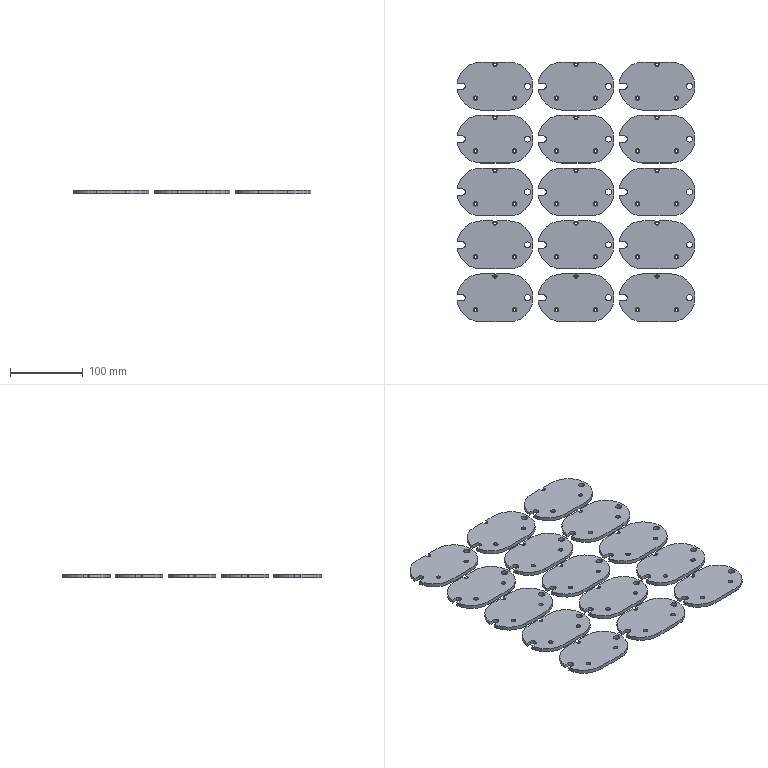NC program | NX | posted with a generic post | part box 328.125 x 358 x 5 mm
Whole program:
N10 G17 G21 G94 G90
(DRILLING , TOOL : D6A45)
N12 T14 M6
N14 G54
N16 G17 G0 G90 X0.137 Y30. S5000 M3
N18 G43 Z30. H14
N20 G94 G81 G98 Z-1.2 F250. R3.
N22 X26.984 Y-16.5
N24 X-26.709
N26 X-44.863 Y0.
N28 G80
N30 G0 X-44.863 Y0. Z30.
N32 M5
(DRILLING_COPY , TOOL : 5.5ZT)
N34 T15 M6
N36 G54
N38 G17 G0 G90 X26.984 Y-16.5 S2000 M3
N40 G43 Z30. H15
N42 G94 G83 G98 Z-4.552 F150. Q2. R3.
N44 X0.137 Y30.
N46 X-26.709 Y-16.5
N48 G80
N50 G0 X-26.709 Y-16.5 Z30.
N52 M5
(DRILLING_COPY_COPY , TOOL : 8.5ZT)
N54 T13 M6
N56 G54
N58 G17 G0 G90 X-44.863 Y0. S2000 M3
N60 G43 Z30. H13
N62 G94 G83 G98 Z-9.054 F150. Q2. R3.
N64 G80
N66 G0 X-44.863 Y0. Z30.
N68 M5
(PLANAR_MILL_COPY , TOOL : D6A45)
N70 T14 M6
N72 G54
N74 G17 G0 G90 X-47.713 Y0.866 S9500 M3
N76 G43 Z30. H14
N78 Z0.
N80 G94 G1 Z-1. F1250.
N82 G3 X-48.213 Y0. R1.
N84 X-44.863 Y-3.35 R3.35
N86 X-48.213 Y0. R-3.35
N88 X-47.713 Y-0.866 R1.
N90 G1 Z0.
N92 G0 Z30.
N94 X-27.142 Y-17.1
N96 Z0.
N98 G1 Z-1.
N100 G3 X-26.709 Y-17.35 R0.5
N102 X-25.859 Y-16.5 R0.85
N104 X-26.709 Y-17.35 R-0.85
N106 X-26.276 Y-17.1 R0.5
N108 G1 Z0.
N110 G0 Z30.
N112 X1.003 Y-34.4
N114 Z0.
N116 G1 Z-1.
N118 G3 X0.137 Y-33.9 R1.
N120 G1 X-19.363
N122 G2 X-53.263 Y0. R33.9
N124 X-19.363 Y33.9 R33.9
N126 G1 X19.637
N128 G2 X53.255 Y4.366 R33.9
N130 X52.363 Y3.35 R0.9
N132 G1 X45.137
N134 G3 X41.787 Y0. R3.35
N136 X45.137 Y-3.35 R3.35
N138 G1 X52.363
N140 G2 X53.255 Y-4.366 R0.9
N142 X19.637 Y-33.9 R33.9
N144 G1 X0.137
N146 G3 X-0.729 Y-34.4 R1.
N148 G1 Z0.
N150 G0 Z30.
N152 X0.57 Y30.6
N154 Z0.
N156 G1 Z-1.
N158 G3 X0.137 Y30.85 R0.5
N160 X-0.713 Y30. R0.85
N162 X0.137 Y30.85 R-0.85
N164 X-0.296 Y30.6 R0.5
N166 G1 Z0.
N168 G0 Z30.
N170 X26.551 Y-17.1
N172 Z0.
N174 G1 Z-1.
N176 G3 X26.984 Y-17.35 R0.5
N178 X27.834 Y-16.5 R0.85
N180 X26.984 Y-17.35 R-0.85
N182 X27.417 Y-17.1 R0.5
N184 G1 Z0.
N186 G0 Z30.
N188 M5
N190 M2